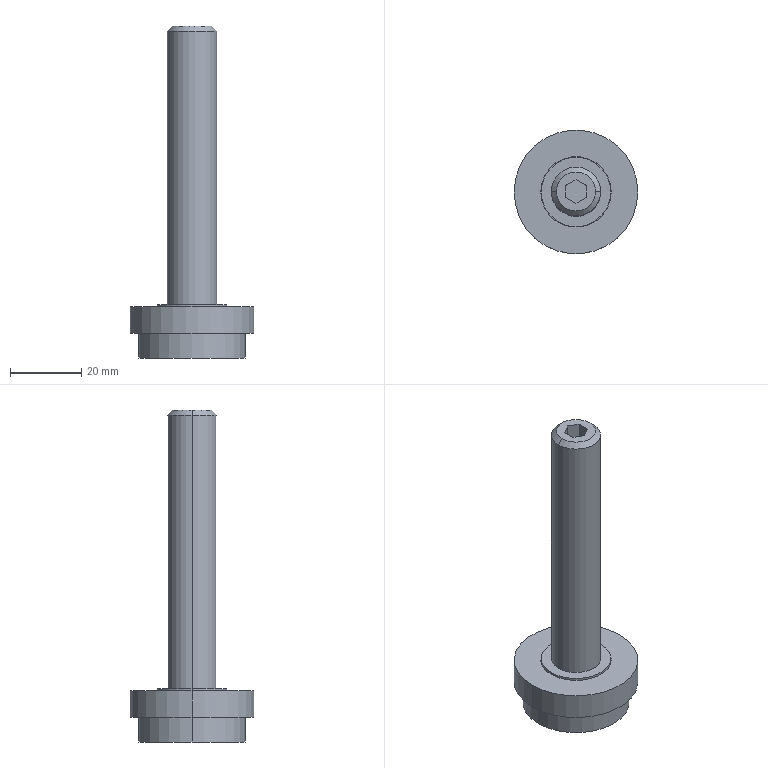Part | SolidWorks | features BaseBody 1 | 1 solid | 25 faces | box 34.846 x 34.846 x 93.462 mm | volume 23774 mm3 | plane 13 | cylinder 10 | cone 2 | commonest cylinder face diameters 13.846 x2 19.615 x2 19.846 x2 30 x2 34.846 x2
STEP:
#1=CARTESIAN_POINT('',(-24.677,360.269,346.277));
#2=VERTEX_POINT('',#1);
#3=CARTESIAN_POINT('',(-10.83,360.269,346.277));
#4=VERTEX_POINT('',#3);
#5=CARTESIAN_POINT('',(-17.753,360.269,346.277));
#6=DIRECTION('',(0.,0.,-1.));
#7=DIRECTION('',(-1.,0.,0.));
#8=AXIS2_PLACEMENT_3D('',#5,#6,#7);
#9=CIRCLE('',#8,6.923);
#10=EDGE_CURVE('',#2,#4,#9,.T.);
#11=ORIENTED_EDGE('',*,*,#10,.T.);
#12=CARTESIAN_POINT('',(-10.83,360.269,269.231));
#13=VERTEX_POINT('',#12);
#14=CARTESIAN_POINT('',(-10.83,360.269,347.692));
#15=DIRECTION('',(0.,0.,-1.));
#16=VECTOR('',#15,1000.);
#17=LINE('',#14,#16);
#18=EDGE_CURVE('',#4,#13,#17,.T.);
#19=ORIENTED_EDGE('',*,*,#18,.T.);
#20=CARTESIAN_POINT('',(-24.677,360.269,269.231));
#21=VERTEX_POINT('',#20);
#22=CARTESIAN_POINT('',(-17.753,360.269,269.231));
#23=DIRECTION('',(0.,0.,1.));
#24=DIRECTION('',(-1.,0.,0.));
#25=AXIS2_PLACEMENT_3D('',#22,#23,#24);
#26=CIRCLE('',#25,6.923);
#27=EDGE_CURVE('',#13,#21,#26,.T.);
#28=ORIENTED_EDGE('',*,*,#27,.T.);
#29=CARTESIAN_POINT('',(-24.677,360.269,347.692));
#30=DIRECTION('',(0.,0.,-1.));
#31=VECTOR('',#30,1000.);
#32=LINE('',#29,#31);
#33=EDGE_CURVE('',#2,#21,#32,.T.);
#34=ORIENTED_EDGE('',*,*,#33,.F.);
#35=EDGE_LOOP('',(#11,#19,#28,#34));
#36=FACE_OUTER_BOUND('',#35,.T.);
#37=CARTESIAN_POINT('',(-17.753,360.269,347.692));
#38=DIRECTION('',(0.,0.,-1.));
#39=DIRECTION('',(-1.,0.,0.));
#40=AXIS2_PLACEMENT_3D('',#37,#38,#39);
#41=CYLINDRICAL_SURFACE('',#40,6.923);
#42=ADVANCED_FACE('',(#36),#41,.T.);
#43=CARTESIAN_POINT('',(-23.261,360.269,347.692));
#44=VERTEX_POINT('',#43);
#45=CARTESIAN_POINT('',(-12.246,360.269,347.692));
#46=VERTEX_POINT('',#45);
#47=CARTESIAN_POINT('',(-17.753,360.269,347.692));
#48=DIRECTION('',(0.,0.,-1.));
#49=DIRECTION('',(-1.,0.,0.));
#50=AXIS2_PLACEMENT_3D('',#47,#48,#49);
#51=CIRCLE('',#50,5.507);
#52=EDGE_CURVE('',#44,#46,#51,.T.);
#53=ORIENTED_EDGE('',*,*,#52,.T.);
#54=CARTESIAN_POINT('',(-10.83,360.269,346.277));
#55=DIRECTION('',(0.7071,0.,-0.7071));
#56=VECTOR('',#55,1000.);
#57=LINE('',#54,#56);
#58=EDGE_CURVE('',#46,#4,#57,.T.);
#59=ORIENTED_EDGE('',*,*,#58,.T.);
#60=ORIENTED_EDGE('',*,*,#10,.F.);
#61=CARTESIAN_POINT('',(-24.677,360.269,346.277));
#62=DIRECTION('',(-0.7071,0.,-0.7071));
#63=VECTOR('',#62,1000.);
#64=LINE('',#61,#63);
#65=EDGE_CURVE('',#44,#2,#64,.T.);
#66=ORIENTED_EDGE('',*,*,#65,.F.);
#67=EDGE_LOOP('',(#53,#59,#60,#66));
#68=FACE_OUTER_BOUND('',#67,.T.);
#69=CARTESIAN_POINT('',(-17.753,360.269,346.277));
#70=DIRECTION('',(0.,0.,-1.));
#71=DIRECTION('',(-1.,0.,0.));
#72=AXIS2_PLACEMENT_3D('',#69,#70,#71);
#73=CONICAL_SURFACE('',#72,6.923,0.7854);
#74=ADVANCED_FACE('',(#68),#73,.T.);
#75=CARTESIAN_POINT('',(-27.561,360.269,269.231));
#76=VERTEX_POINT('',#75);
#77=CARTESIAN_POINT('',(-7.946,360.269,269.231));
#78=VERTEX_POINT('',#77);
#79=CARTESIAN_POINT('',(-17.753,360.269,269.231));
#80=DIRECTION('',(0.,0.,-1.));
#81=DIRECTION('',(-1.,0.,0.));
#82=AXIS2_PLACEMENT_3D('',#79,#80,#81);
#83=CIRCLE('',#82,9.808);
#84=EDGE_CURVE('',#76,#78,#83,.T.);
#85=ORIENTED_EDGE('',*,*,#84,.T.);
#86=CARTESIAN_POINT('',(-7.946,360.269,261.154));
#87=VERTEX_POINT('',#86);
#88=CARTESIAN_POINT('',(-7.946,360.269,347.692));
#89=DIRECTION('',(0.,0.,-1.));
#90=VECTOR('',#89,1000.);
#91=LINE('',#88,#90);
#92=EDGE_CURVE('',#78,#87,#91,.T.);
#93=ORIENTED_EDGE('',*,*,#92,.T.);
#94=CARTESIAN_POINT('',(-27.561,360.269,261.154));
#95=VERTEX_POINT('',#94);
#96=CARTESIAN_POINT('',(-17.753,360.269,261.154));
#97=DIRECTION('',(0.,0.,1.));
#98=DIRECTION('',(-1.,0.,0.));
#99=AXIS2_PLACEMENT_3D('',#96,#97,#98);
#100=CIRCLE('',#99,9.808);
#101=EDGE_CURVE('',#87,#95,#100,.T.);
#102=ORIENTED_EDGE('',*,*,#101,.T.);
#103=CARTESIAN_POINT('',(-27.561,360.269,347.692));
#104=DIRECTION('',(0.,0.,-1.));
#105=VECTOR('',#104,1000.);
#106=LINE('',#103,#105);
#107=EDGE_CURVE('',#76,#95,#106,.T.);
#108=ORIENTED_EDGE('',*,*,#107,.F.);
#109=EDGE_LOOP('',(#85,#93,#102,#108));
#110=FACE_OUTER_BOUND('',#109,.T.);
#111=CARTESIAN_POINT('',(-17.753,360.269,347.692));
#112=DIRECTION('',(0.,0.,-1.));
#113=DIRECTION('',(-1.,0.,0.));
#114=AXIS2_PLACEMENT_3D('',#111,#112,#113);
#115=CYLINDRICAL_SURFACE('',#114,9.808);
#116=ADVANCED_FACE('',(#110),#115,.T.);
#117=CARTESIAN_POINT('',(-7.83,360.269,261.154));
#118=VERTEX_POINT('',#117);
#119=CARTESIAN_POINT('',(-27.677,360.269,261.154));
#120=VERTEX_POINT('',#119);
#121=CARTESIAN_POINT('',(-17.753,360.269,261.154));
#122=DIRECTION('',(0.,0.,-1.));
#123=DIRECTION('',(1.,0.,0.));
#124=AXIS2_PLACEMENT_3D('',#121,#122,#123);
#125=CIRCLE('',#124,9.923);
#126=EDGE_CURVE('',#118,#120,#125,.T.);
#127=ORIENTED_EDGE('',*,*,#126,.T.);
#128=CARTESIAN_POINT('',(-27.677,360.269,268.654));
#129=VERTEX_POINT('',#128);
#130=CARTESIAN_POINT('',(-27.677,360.269,268.654));
#131=DIRECTION('',(0.,0.,1.));
#132=VECTOR('',#131,1000.);
#133=LINE('',#130,#132);
#134=EDGE_CURVE('',#120,#129,#133,.T.);
#135=ORIENTED_EDGE('',*,*,#134,.T.);
#136=CARTESIAN_POINT('',(-7.83,360.269,268.654));
#137=VERTEX_POINT('',#136);
#138=CARTESIAN_POINT('',(-17.753,360.269,268.654));
#139=DIRECTION('',(0.,0.,-1.));
#140=DIRECTION('',(1.,0.,0.));
#141=AXIS2_PLACEMENT_3D('',#138,#139,#140);
#142=CIRCLE('',#141,9.923);
#143=EDGE_CURVE('',#137,#129,#142,.T.);
#144=ORIENTED_EDGE('',*,*,#143,.F.);
#145=CARTESIAN_POINT('',(-7.83,360.269,268.654));
#146=DIRECTION('',(0.,0.,1.));
#147=VECTOR('',#146,1000.);
#148=LINE('',#145,#147);
#149=EDGE_CURVE('',#118,#137,#148,.T.);
#150=ORIENTED_EDGE('',*,*,#149,.F.);
#151=EDGE_LOOP('',(#127,#135,#144,#150));
#152=FACE_OUTER_BOUND('',#151,.T.);
#153=CARTESIAN_POINT('',(-17.753,360.269,268.654));
#154=DIRECTION('',(0.,0.,1.));
#155=DIRECTION('',(1.,0.,0.));
#156=AXIS2_PLACEMENT_3D('',#153,#154,#155);
#157=CYLINDRICAL_SURFACE('',#156,9.923);
#158=ADVANCED_FACE('',(#152),#157,.F.);
#159=CARTESIAN_POINT('',(-0.3304,360.269,261.154));
#160=VERTEX_POINT('',#159);
#161=CARTESIAN_POINT('',(-35.177,360.269,261.154));
#162=VERTEX_POINT('',#161);
#163=CARTESIAN_POINT('',(-17.753,360.269,261.154));
#164=DIRECTION('',(0.,0.,1.));
#165=DIRECTION('',(1.,0.,0.));
#166=AXIS2_PLACEMENT_3D('',#163,#164,#165);
#167=CIRCLE('',#166,17.423);
#168=EDGE_CURVE('',#160,#162,#167,.T.);
#169=ORIENTED_EDGE('',*,*,#168,.T.);
#170=CARTESIAN_POINT('',(-35.177,360.269,268.654));
#171=VERTEX_POINT('',#170);
#172=CARTESIAN_POINT('',(-35.177,360.269,268.654));
#173=DIRECTION('',(0.,0.,1.));
#174=VECTOR('',#173,1000.);
#175=LINE('',#172,#174);
#176=EDGE_CURVE('',#162,#171,#175,.T.);
#177=ORIENTED_EDGE('',*,*,#176,.T.);
#178=CARTESIAN_POINT('',(-0.3304,360.269,268.654));
#179=VERTEX_POINT('',#178);
#180=CARTESIAN_POINT('',(-17.753,360.269,268.654));
#181=DIRECTION('',(0.,0.,1.));
#182=DIRECTION('',(1.,0.,0.));
#183=AXIS2_PLACEMENT_3D('',#180,#181,#182);
#184=CIRCLE('',#183,17.423);
#185=EDGE_CURVE('',#179,#171,#184,.T.);
#186=ORIENTED_EDGE('',*,*,#185,.F.);
#187=CARTESIAN_POINT('',(-0.3304,360.269,268.654));
#188=DIRECTION('',(0.,0.,1.));
#189=VECTOR('',#188,1000.);
#190=LINE('',#187,#189);
#191=EDGE_CURVE('',#160,#179,#190,.T.);
#192=ORIENTED_EDGE('',*,*,#191,.F.);
#193=EDGE_LOOP('',(#169,#177,#186,#192));
#194=FACE_OUTER_BOUND('',#193,.T.);
#195=CARTESIAN_POINT('',(-17.753,360.269,268.654));
#196=DIRECTION('',(0.,0.,1.));
#197=DIRECTION('',(1.,0.,0.));
#198=AXIS2_PLACEMENT_3D('',#195,#196,#197);
#199=CYLINDRICAL_SURFACE('',#198,17.423);
#200=ADVANCED_FACE('',(#194),#199,.T.);
#201=CARTESIAN_POINT('',(-32.753,360.269,261.154));
#202=VERTEX_POINT('',#201);
#203=CARTESIAN_POINT('',(-2.753,360.269,261.154));
#204=VERTEX_POINT('',#203);
#205=CARTESIAN_POINT('',(-17.753,360.269,261.154));
#206=DIRECTION('',(0.,0.,-1.));
#207=DIRECTION('',(-1.,0.,0.));
#208=AXIS2_PLACEMENT_3D('',#205,#206,#207);
#209=CIRCLE('',#208,15.);
#210=EDGE_CURVE('',#202,#204,#209,.T.);
#211=ORIENTED_EDGE('',*,*,#210,.T.);
#212=CARTESIAN_POINT('',(-2.753,360.269,254.231));
#213=VERTEX_POINT('',#212);
#214=CARTESIAN_POINT('',(-2.753,360.269,347.692));
#215=DIRECTION('',(0.,0.,-1.));
#216=VECTOR('',#215,1000.);
#217=LINE('',#214,#216);
#218=EDGE_CURVE('',#204,#213,#217,.T.);
#219=ORIENTED_EDGE('',*,*,#218,.T.);
#220=CARTESIAN_POINT('',(-32.753,360.269,254.231));
#221=VERTEX_POINT('',#220);
#222=CARTESIAN_POINT('',(-17.753,360.269,254.231));
#223=DIRECTION('',(0.,0.,1.));
#224=DIRECTION('',(-1.,0.,0.));
#225=AXIS2_PLACEMENT_3D('',#222,#223,#224);
#226=CIRCLE('',#225,15.);
#227=EDGE_CURVE('',#213,#221,#226,.T.);
#228=ORIENTED_EDGE('',*,*,#227,.T.);
#229=CARTESIAN_POINT('',(-32.753,360.269,347.692));
#230=DIRECTION('',(0.,0.,-1.));
#231=VECTOR('',#230,1000.);
#232=LINE('',#229,#231);
#233=EDGE_CURVE('',#202,#221,#232,.T.);
#234=ORIENTED_EDGE('',*,*,#233,.F.);
#235=EDGE_LOOP('',(#211,#219,#228,#234));
#236=FACE_OUTER_BOUND('',#235,.T.);
#237=CARTESIAN_POINT('',(-17.753,360.269,347.692));
#238=DIRECTION('',(0.,0.,-1.));
#239=DIRECTION('',(-1.,0.,0.));
#240=AXIS2_PLACEMENT_3D('',#237,#238,#239);
#241=CYLINDRICAL_SURFACE('',#240,15.);
#242=ADVANCED_FACE('',(#236),#241,.T.);
#243=ORIENTED_EDGE('',*,*,#18,.F.);
#244=CARTESIAN_POINT('',(-17.753,360.269,346.277));
#245=DIRECTION('',(0.,0.,-1.));
#246=DIRECTION('',(-1.,0.,0.));
#247=AXIS2_PLACEMENT_3D('',#244,#245,#246);
#248=CIRCLE('',#247,6.923);
#249=EDGE_CURVE('',#4,#2,#248,.T.);
#250=ORIENTED_EDGE('',*,*,#249,.T.);
#251=ORIENTED_EDGE('',*,*,#33,.T.);
#252=CARTESIAN_POINT('',(-17.753,360.269,269.231));
#253=DIRECTION('',(0.,0.,1.));
#254=DIRECTION('',(-1.,0.,0.));
#255=AXIS2_PLACEMENT_3D('',#252,#253,#254);
#256=CIRCLE('',#255,6.923);
#257=EDGE_CURVE('',#21,#13,#256,.T.);
#258=ORIENTED_EDGE('',*,*,#257,.T.);
#259=EDGE_LOOP('',(#243,#250,#251,#258));
#260=FACE_OUTER_BOUND('',#259,.T.);
#261=CARTESIAN_POINT('',(-17.753,360.269,347.692));
#262=DIRECTION('',(0.,0.,-1.));
#263=DIRECTION('',(-1.,0.,0.));
#264=AXIS2_PLACEMENT_3D('',#261,#262,#263);
#265=CYLINDRICAL_SURFACE('',#264,6.923);
#266=ADVANCED_FACE('',(#260),#265,.T.);
#267=ORIENTED_EDGE('',*,*,#58,.F.);
#268=CARTESIAN_POINT('',(-17.753,360.269,347.692));
#269=DIRECTION('',(0.,0.,-1.));
#270=DIRECTION('',(-1.,0.,0.));
#271=AXIS2_PLACEMENT_3D('',#268,#269,#270);
#272=CIRCLE('',#271,5.507);
#273=EDGE_CURVE('',#46,#44,#272,.T.);
#274=ORIENTED_EDGE('',*,*,#273,.T.);
#275=ORIENTED_EDGE('',*,*,#65,.T.);
#276=ORIENTED_EDGE('',*,*,#249,.F.);
#277=EDGE_LOOP('',(#267,#274,#275,#276));
#278=FACE_OUTER_BOUND('',#277,.T.);
#279=CARTESIAN_POINT('',(-17.753,360.269,346.277));
#280=DIRECTION('',(0.,0.,-1.));
#281=DIRECTION('',(-1.,0.,0.));
#282=AXIS2_PLACEMENT_3D('',#279,#280,#281);
#283=CONICAL_SURFACE('',#282,6.923,0.7854);
#284=ADVANCED_FACE('',(#278),#283,.T.);
#285=ORIENTED_EDGE('',*,*,#257,.F.);
#286=ORIENTED_EDGE('',*,*,#27,.F.);
#287=EDGE_LOOP('',(#285,#286));
#288=FACE_BOUND('',#287,.T.);
#289=ORIENTED_EDGE('',*,*,#84,.F.);
#290=CARTESIAN_POINT('',(-17.753,360.269,269.231));
#291=DIRECTION('',(0.,0.,-1.));
#292=DIRECTION('',(-1.,0.,0.));
#293=AXIS2_PLACEMENT_3D('',#290,#291,#292);
#294=CIRCLE('',#293,9.808);
#295=EDGE_CURVE('',#78,#76,#294,.T.);
#296=ORIENTED_EDGE('',*,*,#295,.F.);
#297=EDGE_LOOP('',(#289,#296));
#298=FACE_OUTER_BOUND('',#297,.T.);
#299=CARTESIAN_POINT('',(-17.753,350.462,269.231));
#300=DIRECTION('',(0.,0.,-1.));
#301=DIRECTION('',(-1.,0.,0.));
#302=AXIS2_PLACEMENT_3D('',#299,#300,#301);
#303=PLANE('',#302);
#304=ADVANCED_FACE('',(#288,#298),#303,.F.);
#305=CARTESIAN_POINT('',(-17.753,363.6,347.692));
#306=VERTEX_POINT('',#305);
#307=CARTESIAN_POINT('',(-20.638,361.935,347.692));
#308=VERTEX_POINT('',#307);
#309=CARTESIAN_POINT('',(-17.753,363.6,347.692));
#310=DIRECTION('',(-0.866,-0.5,0.));
#311=VECTOR('',#310,1000.);
#312=LINE('',#309,#311);
#313=EDGE_CURVE('',#306,#308,#312,.T.);
#314=ORIENTED_EDGE('',*,*,#313,.F.);
#315=CARTESIAN_POINT('',(-14.869,361.935,347.692));
#316=VERTEX_POINT('',#315);
#317=CARTESIAN_POINT('',(-14.869,361.935,347.692));
#318=DIRECTION('',(-0.866,0.5,0.));
#319=VECTOR('',#318,1000.);
#320=LINE('',#317,#319);
#321=EDGE_CURVE('',#316,#306,#320,.T.);
#322=ORIENTED_EDGE('',*,*,#321,.F.);
#323=CARTESIAN_POINT('',(-14.869,358.604,347.692));
#324=VERTEX_POINT('',#323);
#325=CARTESIAN_POINT('',(-14.869,354.762,347.692));
#326=DIRECTION('',(0.,1.,0.));
#327=VECTOR('',#326,1000.);
#328=LINE('',#325,#327);
#329=EDGE_CURVE('',#324,#316,#328,.T.);
#330=ORIENTED_EDGE('',*,*,#329,.F.);
#331=CARTESIAN_POINT('',(-17.753,356.938,347.692));
#332=VERTEX_POINT('',#331);
#333=CARTESIAN_POINT('',(-17.753,356.938,347.692));
#334=DIRECTION('',(0.866,0.5,0.));
#335=VECTOR('',#334,1000.);
#336=LINE('',#333,#335);
#337=EDGE_CURVE('',#332,#324,#336,.T.);
#338=ORIENTED_EDGE('',*,*,#337,.F.);
#339=CARTESIAN_POINT('',(-20.638,358.604,347.692));
#340=VERTEX_POINT('',#339);
#341=CARTESIAN_POINT('',(-20.638,358.604,347.692));
#342=DIRECTION('',(0.866,-0.5,0.));
#343=VECTOR('',#342,1000.);
#344=LINE('',#341,#343);
#345=EDGE_CURVE('',#340,#332,#344,.T.);
#346=ORIENTED_EDGE('',*,*,#345,.F.);
#347=CARTESIAN_POINT('',(-20.638,354.762,347.692));
#348=DIRECTION('',(0.,-1.,0.));
#349=VECTOR('',#348,1000.);
#350=LINE('',#347,#349);
#351=EDGE_CURVE('',#308,#340,#350,.T.);
#352=ORIENTED_EDGE('',*,*,#351,.F.);
#353=EDGE_LOOP('',(#314,#322,#330,#338,#346,#352));
#354=FACE_BOUND('',#353,.T.);
#355=ORIENTED_EDGE('',*,*,#52,.F.);
#356=ORIENTED_EDGE('',*,*,#273,.F.);
#357=EDGE_LOOP('',(#355,#356));
#358=FACE_OUTER_BOUND('',#357,.T.);
#359=CARTESIAN_POINT('',(-17.753,354.762,347.692));
#360=DIRECTION('',(0.,0.,-1.));
#361=DIRECTION('',(-1.,0.,0.));
#362=AXIS2_PLACEMENT_3D('',#359,#360,#361);
#363=PLANE('',#362);
#364=ADVANCED_FACE('',(#354,#358),#363,.F.);
#365=ORIENTED_EDGE('',*,*,#92,.F.);
#366=ORIENTED_EDGE('',*,*,#295,.T.);
#367=ORIENTED_EDGE('',*,*,#107,.T.);
#368=CARTESIAN_POINT('',(-17.753,360.269,261.154));
#369=DIRECTION('',(0.,0.,1.));
#370=DIRECTION('',(-1.,0.,0.));
#371=AXIS2_PLACEMENT_3D('',#368,#369,#370);
#372=CIRCLE('',#371,9.808);
#373=EDGE_CURVE('',#95,#87,#372,.T.);
#374=ORIENTED_EDGE('',*,*,#373,.T.);
#375=EDGE_LOOP('',(#365,#366,#367,#374));
#376=FACE_OUTER_BOUND('',#375,.T.);
#377=CARTESIAN_POINT('',(-17.753,360.269,347.692));
#378=DIRECTION('',(0.,0.,-1.));
#379=DIRECTION('',(-1.,0.,0.));
#380=AXIS2_PLACEMENT_3D('',#377,#378,#379);
#381=CYLINDRICAL_SURFACE('',#380,9.808);
#382=ADVANCED_FACE('',(#376),#381,.T.);
#383=CARTESIAN_POINT('',(-20.638,361.935,341.923));
#384=VERTEX_POINT('',#383);
#385=CARTESIAN_POINT('',(-20.638,361.935,341.923));
#386=DIRECTION('',(0.,0.,-1.));
#387=VECTOR('',#386,1000.);
#388=LINE('',#385,#387);
#389=EDGE_CURVE('',#308,#384,#388,.T.);
#390=ORIENTED_EDGE('',*,*,#389,.F.);
#391=ORIENTED_EDGE('',*,*,#351,.T.);
#392=CARTESIAN_POINT('',(-20.638,358.604,341.923));
#393=VERTEX_POINT('',#392);
#394=CARTESIAN_POINT('',(-20.638,358.604,341.923));
#395=DIRECTION('',(0.,0.,1.));
#396=VECTOR('',#395,1000.);
#397=LINE('',#394,#396);
#398=EDGE_CURVE('',#393,#340,#397,.T.);
#399=ORIENTED_EDGE('',*,*,#398,.F.);
#400=CARTESIAN_POINT('',(-20.638,361.935,341.923));
#401=DIRECTION('',(0.,-1.,0.));
#402=VECTOR('',#401,1000.);
#403=LINE('',#400,#402);
#404=EDGE_CURVE('',#384,#393,#403,.T.);
#405=ORIENTED_EDGE('',*,*,#404,.F.);
#406=EDGE_LOOP('',(#390,#391,#399,#405));
#407=FACE_OUTER_BOUND('',#406,.T.);
#408=CARTESIAN_POINT('',(-20.638,361.935,341.923));
#409=DIRECTION('',(-1.,0.,0.));
#410=DIRECTION('',(0.,0.,1.));
#411=AXIS2_PLACEMENT_3D('',#408,#409,#410);
#412=PLANE('',#411);
#413=ADVANCED_FACE('',(#407),#412,.F.);
#414=CARTESIAN_POINT('',(-17.753,363.6,341.923));
#415=VERTEX_POINT('',#414);
#416=CARTESIAN_POINT('',(-17.753,363.6,341.923));
#417=DIRECTION('',(0.,0.,-1.));
#418=VECTOR('',#417,1000.);
#419=LINE('',#416,#418);
#420=EDGE_CURVE('',#306,#415,#419,.T.);
#421=ORIENTED_EDGE('',*,*,#420,.F.);
#422=ORIENTED_EDGE('',*,*,#313,.T.);
#423=ORIENTED_EDGE('',*,*,#389,.T.);
#424=CARTESIAN_POINT('',(-17.753,363.6,341.923));
#425=DIRECTION('',(-0.866,-0.5,0.));
#426=VECTOR('',#425,1000.);
#427=LINE('',#424,#426);
#428=EDGE_CURVE('',#415,#384,#427,.T.);
#429=ORIENTED_EDGE('',*,*,#428,.F.);
#430=EDGE_LOOP('',(#421,#422,#423,#429));
#431=FACE_OUTER_BOUND('',#430,.T.);
#432=CARTESIAN_POINT('',(-17.753,363.6,341.923));
#433=DIRECTION('',(-0.5,0.866,0.));
#434=DIRECTION('',(-0.866,-0.5,0.));
#435=AXIS2_PLACEMENT_3D('',#432,#433,#434);
#436=PLANE('',#435);
#437=ADVANCED_FACE('',(#431),#436,.F.);
#438=CARTESIAN_POINT('',(-14.869,361.935,341.923));
#439=VERTEX_POINT('',#438);
#440=CARTESIAN_POINT('',(-14.869,361.935,341.923));
#441=DIRECTION('',(0.,0.,-1.));
#442=VECTOR('',#441,1000.);
#443=LINE('',#440,#442);
#444=EDGE_CURVE('',#316,#439,#443,.T.);
#445=ORIENTED_EDGE('',*,*,#444,.F.);
#446=ORIENTED_EDGE('',*,*,#321,.T.);
#447=ORIENTED_EDGE('',*,*,#420,.T.);
#448=CARTESIAN_POINT('',(-14.869,361.935,341.923));
#449=DIRECTION('',(-0.866,0.5,0.));
#450=VECTOR('',#449,1000.);
#451=LINE('',#448,#450);
#452=EDGE_CURVE('',#439,#415,#451,.T.);
#453=ORIENTED_EDGE('',*,*,#452,.F.);
#454=EDGE_LOOP('',(#445,#446,#447,#453));
#455=FACE_OUTER_BOUND('',#454,.T.);
#456=CARTESIAN_POINT('',(-14.869,361.935,341.923));
#457=DIRECTION('',(0.5,0.866,0.));
#458=DIRECTION('',(-0.866,0.5,0.));
#459=AXIS2_PLACEMENT_3D('',#456,#457,#458);
#460=PLANE('',#459);
#461=ADVANCED_FACE('',(#455),#460,.F.);
#462=CARTESIAN_POINT('',(-14.869,358.604,341.923));
#463=VERTEX_POINT('',#462);
#464=CARTESIAN_POINT('',(-14.869,358.604,341.923));
#465=DIRECTION('',(0.,0.,-1.));
#466=VECTOR('',#465,1000.);
#467=LINE('',#464,#466);
#468=EDGE_CURVE('',#324,#463,#467,.T.);
#469=ORIENTED_EDGE('',*,*,#468,.F.);
#470=ORIENTED_EDGE('',*,*,#329,.T.);
#471=ORIENTED_EDGE('',*,*,#444,.T.);
#472=CARTESIAN_POINT('',(-14.869,358.604,341.923));
#473=DIRECTION('',(0.,1.,0.));
#474=VECTOR('',#473,1000.);
#475=LINE('',#472,#474);
#476=EDGE_CURVE('',#463,#439,#475,.T.);
#477=ORIENTED_EDGE('',*,*,#476,.F.);
#478=EDGE_LOOP('',(#469,#470,#471,#477));
#479=FACE_OUTER_BOUND('',#478,.T.);
#480=CARTESIAN_POINT('',(-14.869,358.604,341.923));
#481=DIRECTION('',(1.,0.,0.));
#482=DIRECTION('',(0.,0.,-1.));
#483=AXIS2_PLACEMENT_3D('',#480,#481,#482);
#484=PLANE('',#483);
#485=ADVANCED_FACE('',(#479),#484,.F.);
#486=CARTESIAN_POINT('',(-17.753,356.938,341.923));
#487=VERTEX_POINT('',#486);
#488=CARTESIAN_POINT('',(-17.753,356.938,341.923));
#489=DIRECTION('',(0.,0.,-1.));
#490=VECTOR('',#489,1000.);
#491=LINE('',#488,#490);
#492=EDGE_CURVE('',#332,#487,#491,.T.);
#493=ORIENTED_EDGE('',*,*,#492,.F.);
#494=ORIENTED_EDGE('',*,*,#337,.T.);
#495=ORIENTED_EDGE('',*,*,#468,.T.);
#496=CARTESIAN_POINT('',(-17.753,356.938,341.923));
#497=DIRECTION('',(0.866,0.5,0.));
#498=VECTOR('',#497,1000.);
#499=LINE('',#496,#498);
#500=EDGE_CURVE('',#487,#463,#499,.T.);
#501=ORIENTED_EDGE('',*,*,#500,.F.);
#502=EDGE_LOOP('',(#493,#494,#495,#501));
#503=FACE_OUTER_BOUND('',#502,.T.);
#504=CARTESIAN_POINT('',(-17.753,356.938,341.923));
#505=DIRECTION('',(0.5,-0.866,0.));
#506=DIRECTION('',(0.866,0.5,0.));
#507=AXIS2_PLACEMENT_3D('',#504,#505,#506);
#508=PLANE('',#507);
#509=ADVANCED_FACE('',(#503),#508,.F.);
#510=ORIENTED_EDGE('',*,*,#398,.T.);
#511=ORIENTED_EDGE('',*,*,#345,.T.);
#512=ORIENTED_EDGE('',*,*,#492,.T.);
#513=CARTESIAN_POINT('',(-20.638,358.604,341.923));
#514=DIRECTION('',(0.866,-0.5,0.));
#515=VECTOR('',#514,1000.);
#516=LINE('',#513,#515);
#517=EDGE_CURVE('',#393,#487,#516,.T.);
#518=ORIENTED_EDGE('',*,*,#517,.F.);
#519=EDGE_LOOP('',(#510,#511,#512,#518));
#520=FACE_OUTER_BOUND('',#519,.T.);
#521=CARTESIAN_POINT('',(-20.638,358.604,341.923));
#522=DIRECTION('',(-0.5,-0.866,0.));
#523=DIRECTION('',(0.866,-0.5,0.));
#524=AXIS2_PLACEMENT_3D('',#521,#522,#523);
#525=PLANE('',#524);
#526=ADVANCED_FACE('',(#520),#525,.F.);
#527=ORIENTED_EDGE('',*,*,#373,.F.);
#528=ORIENTED_EDGE('',*,*,#101,.F.);
#529=EDGE_LOOP('',(#527,#528));
#530=FACE_BOUND('',#529,.T.);
#531=ORIENTED_EDGE('',*,*,#126,.F.);
#532=CARTESIAN_POINT('',(-17.753,360.269,261.154));
#533=DIRECTION('',(0.,0.,-1.));
#534=DIRECTION('',(1.,0.,0.));
#535=AXIS2_PLACEMENT_3D('',#532,#533,#534);
#536=CIRCLE('',#535,9.923);
#537=EDGE_CURVE('',#120,#118,#536,.T.);
#538=ORIENTED_EDGE('',*,*,#537,.F.);
#539=EDGE_LOOP('',(#531,#538));
#540=FACE_OUTER_BOUND('',#539,.T.);
#541=CARTESIAN_POINT('',(-17.753,345.269,261.154));
#542=DIRECTION('',(0.,0.,-1.));
#543=DIRECTION('',(-1.,0.,0.));
#544=AXIS2_PLACEMENT_3D('',#541,#542,#543);
#545=PLANE('',#544);
#546=ADVANCED_FACE('',(#530,#540),#545,.F.);
#547=ORIENTED_EDGE('',*,*,#428,.T.);
#548=ORIENTED_EDGE('',*,*,#404,.T.);
#549=ORIENTED_EDGE('',*,*,#517,.T.);
#550=ORIENTED_EDGE('',*,*,#500,.T.);
#551=ORIENTED_EDGE('',*,*,#476,.T.);
#552=ORIENTED_EDGE('',*,*,#452,.T.);
#553=EDGE_LOOP('',(#547,#548,#549,#550,#551,#552));
#554=FACE_OUTER_BOUND('',#553,.T.);
#555=CARTESIAN_POINT('',(-17.753,360.269,341.923));
#556=DIRECTION('',(0.,0.,1.));
#557=DIRECTION('',(1.,0.,0.));
#558=AXIS2_PLACEMENT_3D('',#555,#556,#557);
#559=PLANE('',#558);
#560=ADVANCED_FACE('',(#554),#559,.T.);
#561=ORIENTED_EDGE('',*,*,#134,.F.);
#562=ORIENTED_EDGE('',*,*,#537,.T.);
#563=ORIENTED_EDGE('',*,*,#149,.T.);
#564=CARTESIAN_POINT('',(-17.753,360.269,268.654));
#565=DIRECTION('',(0.,0.,-1.));
#566=DIRECTION('',(1.,0.,0.));
#567=AXIS2_PLACEMENT_3D('',#564,#565,#566);
#568=CIRCLE('',#567,9.923);
#569=EDGE_CURVE('',#129,#137,#568,.T.);
#570=ORIENTED_EDGE('',*,*,#569,.F.);
#571=EDGE_LOOP('',(#561,#562,#563,#570));
#572=FACE_OUTER_BOUND('',#571,.T.);
#573=CARTESIAN_POINT('',(-17.753,360.269,268.654));
#574=DIRECTION('',(0.,0.,1.));
#575=DIRECTION('',(1.,0.,0.));
#576=AXIS2_PLACEMENT_3D('',#573,#574,#575);
#577=CYLINDRICAL_SURFACE('',#576,9.923);
#578=ADVANCED_FACE('',(#572),#577,.F.);
#579=ORIENTED_EDGE('',*,*,#143,.T.);
#580=ORIENTED_EDGE('',*,*,#569,.T.);
#581=EDGE_LOOP('',(#579,#580));
#582=FACE_BOUND('',#581,.T.);
#583=ORIENTED_EDGE('',*,*,#185,.T.);
#584=CARTESIAN_POINT('',(-17.753,360.269,268.654));
#585=DIRECTION('',(0.,0.,1.));
#586=DIRECTION('',(1.,0.,0.));
#587=AXIS2_PLACEMENT_3D('',#584,#585,#586);
#588=CIRCLE('',#587,17.423);
#589=EDGE_CURVE('',#171,#179,#588,.T.);
#590=ORIENTED_EDGE('',*,*,#589,.T.);
#591=EDGE_LOOP('',(#583,#590));
#592=FACE_OUTER_BOUND('',#591,.T.);
#593=CARTESIAN_POINT('',(-17.753,360.269,268.654));
#594=DIRECTION('',(0.,0.,1.));
#595=DIRECTION('',(1.,0.,0.));
#596=AXIS2_PLACEMENT_3D('',#593,#594,#595);
#597=PLANE('',#596);
#598=ADVANCED_FACE('',(#582,#592),#597,.T.);
#599=ORIENTED_EDGE('',*,*,#176,.F.);
#600=CARTESIAN_POINT('',(-17.753,360.269,261.154));
#601=DIRECTION('',(0.,0.,1.));
#602=DIRECTION('',(1.,0.,0.));
#603=AXIS2_PLACEMENT_3D('',#600,#601,#602);
#604=CIRCLE('',#603,17.423);
#605=EDGE_CURVE('',#162,#160,#604,.T.);
#606=ORIENTED_EDGE('',*,*,#605,.T.);
#607=ORIENTED_EDGE('',*,*,#191,.T.);
#608=ORIENTED_EDGE('',*,*,#589,.F.);
#609=EDGE_LOOP('',(#599,#606,#607,#608));
#610=FACE_OUTER_BOUND('',#609,.T.);
#611=CARTESIAN_POINT('',(-17.753,360.269,268.654));
#612=DIRECTION('',(0.,0.,1.));
#613=DIRECTION('',(1.,0.,0.));
#614=AXIS2_PLACEMENT_3D('',#611,#612,#613);
#615=CYLINDRICAL_SURFACE('',#614,17.423);
#616=ADVANCED_FACE('',(#610),#615,.T.);
#617=ORIENTED_EDGE('',*,*,#210,.F.);
#618=CARTESIAN_POINT('',(-17.753,360.269,261.154));
#619=DIRECTION('',(0.,0.,-1.));
#620=DIRECTION('',(-1.,0.,0.));
#621=AXIS2_PLACEMENT_3D('',#618,#619,#620);
#622=CIRCLE('',#621,15.);
#623=EDGE_CURVE('',#204,#202,#622,.T.);
#624=ORIENTED_EDGE('',*,*,#623,.F.);
#625=EDGE_LOOP('',(#617,#624));
#626=FACE_BOUND('',#625,.T.);
#627=ORIENTED_EDGE('',*,*,#168,.F.);
#628=ORIENTED_EDGE('',*,*,#605,.F.);
#629=EDGE_LOOP('',(#627,#628));
#630=FACE_OUTER_BOUND('',#629,.T.);
#631=CARTESIAN_POINT('',(-17.753,360.269,261.154));
#632=DIRECTION('',(0.,0.,1.));
#633=DIRECTION('',(1.,0.,0.));
#634=AXIS2_PLACEMENT_3D('',#631,#632,#633);
#635=PLANE('',#634);
#636=ADVANCED_FACE('',(#626,#630),#635,.F.);
#637=ORIENTED_EDGE('',*,*,#218,.F.);
#638=ORIENTED_EDGE('',*,*,#623,.T.);
#639=ORIENTED_EDGE('',*,*,#233,.T.);
#640=CARTESIAN_POINT('',(-17.753,360.269,254.231));
#641=DIRECTION('',(0.,0.,1.));
#642=DIRECTION('',(-1.,0.,0.));
#643=AXIS2_PLACEMENT_3D('',#640,#641,#642);
#644=CIRCLE('',#643,15.);
#645=EDGE_CURVE('',#221,#213,#644,.T.);
#646=ORIENTED_EDGE('',*,*,#645,.T.);
#647=EDGE_LOOP('',(#637,#638,#639,#646));
#648=FACE_OUTER_BOUND('',#647,.T.);
#649=CARTESIAN_POINT('',(-17.753,360.269,347.692));
#650=DIRECTION('',(0.,0.,-1.));
#651=DIRECTION('',(-1.,0.,0.));
#652=AXIS2_PLACEMENT_3D('',#649,#650,#651);
#653=CYLINDRICAL_SURFACE('',#652,15.);
#654=ADVANCED_FACE('',(#648),#653,.T.);
#655=ORIENTED_EDGE('',*,*,#645,.F.);
#656=ORIENTED_EDGE('',*,*,#227,.F.);
#657=EDGE_LOOP('',(#655,#656));
#658=FACE_OUTER_BOUND('',#657,.T.);
#659=CARTESIAN_POINT('',(-17.753,360.269,254.231));
#660=DIRECTION('',(0.,0.,1.));
#661=DIRECTION('',(1.,0.,0.));
#662=AXIS2_PLACEMENT_3D('',#659,#660,#661);
#663=PLANE('',#662);
#664=ADVANCED_FACE('',(#658),#663,.F.);
#665=CLOSED_SHELL('',(#42,#74,#116,#158,#200,#242,#266,#284,#304,#364,#382,#413,#437,#461,#485,#509,#526,#546,#560,#578,#598,#616,#636,#654,#664));
#666=MANIFOLD_SOLID_BREP('',#665);
#667=CARTESIAN_POINT('',(0.,0.,0.));
#668=DIRECTION('',(0.,0.,1.));
#669=DIRECTION('',(1.,0.,0.));
#670=AXIS2_PLACEMENT_3D('',#667,#668,#669);
#671=(LENGTH_UNIT()NAMED_UNIT(*)SI_UNIT(.MILLI.,.METRE.));
#672=UNCERTAINTY_MEASURE_WITH_UNIT(LENGTH_MEASURE(0.00001),#671,'','');
#673=(NAMED_UNIT(*)PLANE_ANGLE_UNIT()SI_UNIT($,.RADIAN.));
#674=(NAMED_UNIT(*)SI_UNIT($,.STERADIAN.)SOLID_ANGLE_UNIT());
#675=(GEOMETRIC_REPRESENTATION_CONTEXT(3)GLOBAL_UNCERTAINTY_ASSIGNED_CONTEXT((#672))GLOBAL_UNIT_ASSIGNED_CONTEXT((#671,#673,#674))REPRESENTATION_CONTEXT('',''));
#676=ADVANCED_BREP_SHAPE_REPRESENTATION('',(#666,#670),#675);